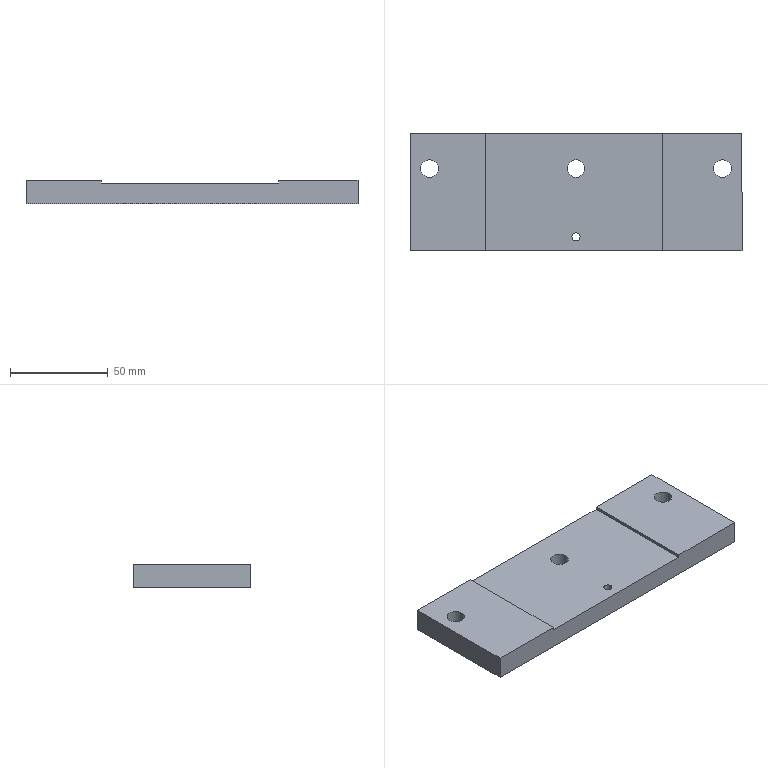Part | SolidWorks | features ICE 2, 3DProfileFeature 1, Extrusion 1, HoleWzd 1 | 1 solid | 20 faces | box 170 x 60 x 12 mm | volume 111868 mm3 | plane 10 | cylinder 8 | cone 2 | commonest cylinder face diameters 9 x6 4.2 x2
STEP:
#1=CARTESIAN_POINT('',(2.1,-23.,-5.575));
#2=VERTEX_POINT('',#1);
#3=CARTESIAN_POINT('',(-2.1,-23.,-5.575));
#4=VERTEX_POINT('',#3);
#5=CARTESIAN_POINT('',(0.,-23.,-5.575));
#6=DIRECTION('',(0.,0.,-1.));
#7=DIRECTION('',(-1.,0.,0.));
#8=AXIS2_PLACEMENT_3D('',#5,#6,#7);
#9=CIRCLE('',#8,2.1);
#10=EDGE_CURVE('',#2,#4,#9,.T.);
#11=ORIENTED_EDGE('',*,*,#10,.F.);
#12=CARTESIAN_POINT('',(2.525,-23.,-6.));
#13=VERTEX_POINT('',#12);
#14=CARTESIAN_POINT('',(2.525,-23.,-6.));
#15=DIRECTION('',(0.7071,0.,-0.7071));
#16=VECTOR('',#15,1000.);
#17=LINE('',#14,#16);
#18=EDGE_CURVE('',#2,#13,#17,.T.);
#19=ORIENTED_EDGE('',*,*,#18,.T.);
#20=CARTESIAN_POINT('',(-2.525,-23.,-6.));
#21=VERTEX_POINT('',#20);
#22=CARTESIAN_POINT('',(0.,-23.,-6.));
#23=DIRECTION('',(0.,0.,-1.));
#24=DIRECTION('',(-1.,0.,0.));
#25=AXIS2_PLACEMENT_3D('',#22,#23,#24);
#26=CIRCLE('',#25,2.525);
#27=EDGE_CURVE('',#13,#21,#26,.T.);
#28=ORIENTED_EDGE('',*,*,#27,.T.);
#29=CARTESIAN_POINT('',(-2.525,-23.,-6.));
#30=DIRECTION('',(-0.7071,0.,-0.7071));
#31=VECTOR('',#30,1000.);
#32=LINE('',#29,#31);
#33=EDGE_CURVE('',#4,#21,#32,.T.);
#34=ORIENTED_EDGE('',*,*,#33,.F.);
#35=EDGE_LOOP('',(#11,#19,#28,#34));
#36=FACE_OUTER_BOUND('',#35,.T.);
#37=CARTESIAN_POINT('',(0.,-23.,-6.));
#38=DIRECTION('',(0.,0.,-1.));
#39=DIRECTION('',(-1.,0.,0.));
#40=AXIS2_PLACEMENT_3D('',#37,#38,#39);
#41=CONICAL_SURFACE('',#40,2.525,0.7854);
#42=ADVANCED_FACE('',(#36),#41,.F.);
#43=CARTESIAN_POINT('',(2.1,-23.,4.5));
#44=VERTEX_POINT('',#43);
#45=CARTESIAN_POINT('',(-2.1,-23.,4.5));
#46=VERTEX_POINT('',#45);
#47=CARTESIAN_POINT('',(0.,-23.,4.5));
#48=DIRECTION('',(0.,0.,-1.));
#49=DIRECTION('',(-1.,0.,0.));
#50=AXIS2_PLACEMENT_3D('',#47,#48,#49);
#51=CIRCLE('',#50,2.1);
#52=EDGE_CURVE('',#44,#46,#51,.T.);
#53=ORIENTED_EDGE('',*,*,#52,.F.);
#54=CARTESIAN_POINT('',(2.1,-23.,-6.));
#55=DIRECTION('',(0.,0.,-1.));
#56=VECTOR('',#55,1000.);
#57=LINE('',#54,#56);
#58=EDGE_CURVE('',#44,#2,#57,.T.);
#59=ORIENTED_EDGE('',*,*,#58,.T.);
#60=ORIENTED_EDGE('',*,*,#10,.T.);
#61=CARTESIAN_POINT('',(-2.1,-23.,-6.));
#62=DIRECTION('',(0.,0.,-1.));
#63=VECTOR('',#62,1000.);
#64=LINE('',#61,#63);
#65=EDGE_CURVE('',#46,#4,#64,.T.);
#66=ORIENTED_EDGE('',*,*,#65,.F.);
#67=EDGE_LOOP('',(#53,#59,#60,#66));
#68=FACE_OUTER_BOUND('',#67,.T.);
#69=CARTESIAN_POINT('',(0.,-23.,-6.));
#70=DIRECTION('',(0.,0.,-1.));
#71=DIRECTION('',(-1.,0.,0.));
#72=AXIS2_PLACEMENT_3D('',#69,#70,#71);
#73=CYLINDRICAL_SURFACE('',#72,2.1);
#74=ADVANCED_FACE('',(#68),#73,.F.);
#75=CARTESIAN_POINT('',(4.5,12.,4.5));
#76=VERTEX_POINT('',#75);
#77=CARTESIAN_POINT('',(-4.5,12.,4.5));
#78=VERTEX_POINT('',#77);
#79=CARTESIAN_POINT('',(0.,12.,4.5));
#80=DIRECTION('',(0.,0.,-1.));
#81=DIRECTION('',(-1.,0.,0.));
#82=AXIS2_PLACEMENT_3D('',#79,#80,#81);
#83=CIRCLE('',#82,4.5);
#84=EDGE_CURVE('',#76,#78,#83,.T.);
#85=ORIENTED_EDGE('',*,*,#84,.F.);
#86=CARTESIAN_POINT('',(4.5,12.,-6.));
#87=VERTEX_POINT('',#86);
#88=CARTESIAN_POINT('',(4.5,12.,6.));
#89=DIRECTION('',(0.,0.,-1.));
#90=VECTOR('',#89,1000.);
#91=LINE('',#88,#90);
#92=EDGE_CURVE('',#76,#87,#91,.T.);
#93=ORIENTED_EDGE('',*,*,#92,.T.);
#94=CARTESIAN_POINT('',(-4.5,12.,-6.));
#95=VERTEX_POINT('',#94);
#96=CARTESIAN_POINT('',(0.,12.,-6.));
#97=DIRECTION('',(0.,0.,1.));
#98=DIRECTION('',(1.,0.,0.));
#99=AXIS2_PLACEMENT_3D('',#96,#97,#98);
#100=CIRCLE('',#99,4.5);
#101=EDGE_CURVE('',#95,#87,#100,.T.);
#102=ORIENTED_EDGE('',*,*,#101,.F.);
#103=CARTESIAN_POINT('',(-4.5,12.,6.));
#104=DIRECTION('',(0.,0.,-1.));
#105=VECTOR('',#104,1000.);
#106=LINE('',#103,#105);
#107=EDGE_CURVE('',#78,#95,#106,.T.);
#108=ORIENTED_EDGE('',*,*,#107,.F.);
#109=EDGE_LOOP('',(#85,#93,#102,#108));
#110=FACE_OUTER_BOUND('',#109,.T.);
#111=CARTESIAN_POINT('',(0.,12.,6.));
#112=DIRECTION('',(0.,0.,-1.));
#113=DIRECTION('',(-1.,0.,0.));
#114=AXIS2_PLACEMENT_3D('',#111,#112,#113);
#115=CYLINDRICAL_SURFACE('',#114,4.5);
#116=ADVANCED_FACE('',(#110),#115,.F.);
#117=CARTESIAN_POINT('',(70.5,12.,6.));
#118=VERTEX_POINT('',#117);
#119=CARTESIAN_POINT('',(79.5,12.,6.));
#120=VERTEX_POINT('',#119);
#121=CARTESIAN_POINT('',(75.,12.,6.));
#122=DIRECTION('',(0.,0.,1.));
#123=DIRECTION('',(1.,0.,0.));
#124=AXIS2_PLACEMENT_3D('',#121,#122,#123);
#125=CIRCLE('',#124,4.5);
#126=EDGE_CURVE('',#118,#120,#125,.T.);
#127=ORIENTED_EDGE('',*,*,#126,.T.);
#128=CARTESIAN_POINT('',(79.5,12.,-6.));
#129=VERTEX_POINT('',#128);
#130=CARTESIAN_POINT('',(79.5,12.,6.));
#131=DIRECTION('',(0.,0.,-1.));
#132=VECTOR('',#131,1000.);
#133=LINE('',#130,#132);
#134=EDGE_CURVE('',#120,#129,#133,.T.);
#135=ORIENTED_EDGE('',*,*,#134,.T.);
#136=CARTESIAN_POINT('',(70.5,12.,-6.));
#137=VERTEX_POINT('',#136);
#138=CARTESIAN_POINT('',(75.,12.,-6.));
#139=DIRECTION('',(0.,0.,1.));
#140=DIRECTION('',(1.,0.,0.));
#141=AXIS2_PLACEMENT_3D('',#138,#139,#140);
#142=CIRCLE('',#141,4.5);
#143=EDGE_CURVE('',#137,#129,#142,.T.);
#144=ORIENTED_EDGE('',*,*,#143,.F.);
#145=CARTESIAN_POINT('',(70.5,12.,6.));
#146=DIRECTION('',(0.,0.,-1.));
#147=VECTOR('',#146,1000.);
#148=LINE('',#145,#147);
#149=EDGE_CURVE('',#118,#137,#148,.T.);
#150=ORIENTED_EDGE('',*,*,#149,.F.);
#151=EDGE_LOOP('',(#127,#135,#144,#150));
#152=FACE_OUTER_BOUND('',#151,.T.);
#153=CARTESIAN_POINT('',(75.,12.,6.));
#154=DIRECTION('',(0.,0.,-1.));
#155=DIRECTION('',(-1.,0.,0.));
#156=AXIS2_PLACEMENT_3D('',#153,#154,#155);
#157=CYLINDRICAL_SURFACE('',#156,4.5);
#158=ADVANCED_FACE('',(#152),#157,.F.);
#159=CARTESIAN_POINT('',(-79.5,12.,6.));
#160=VERTEX_POINT('',#159);
#161=CARTESIAN_POINT('',(-70.5,12.,6.));
#162=VERTEX_POINT('',#161);
#163=CARTESIAN_POINT('',(-75.,12.,6.));
#164=DIRECTION('',(0.,0.,1.));
#165=DIRECTION('',(1.,0.,0.));
#166=AXIS2_PLACEMENT_3D('',#163,#164,#165);
#167=CIRCLE('',#166,4.5);
#168=EDGE_CURVE('',#160,#162,#167,.T.);
#169=ORIENTED_EDGE('',*,*,#168,.T.);
#170=CARTESIAN_POINT('',(-70.5,12.,-6.));
#171=VERTEX_POINT('',#170);
#172=CARTESIAN_POINT('',(-70.5,12.,6.));
#173=DIRECTION('',(0.,0.,-1.));
#174=VECTOR('',#173,1000.);
#175=LINE('',#172,#174);
#176=EDGE_CURVE('',#162,#171,#175,.T.);
#177=ORIENTED_EDGE('',*,*,#176,.T.);
#178=CARTESIAN_POINT('',(-79.5,12.,-6.));
#179=VERTEX_POINT('',#178);
#180=CARTESIAN_POINT('',(-75.,12.,-6.));
#181=DIRECTION('',(0.,0.,1.));
#182=DIRECTION('',(1.,0.,0.));
#183=AXIS2_PLACEMENT_3D('',#180,#181,#182);
#184=CIRCLE('',#183,4.5);
#185=EDGE_CURVE('',#179,#171,#184,.T.);
#186=ORIENTED_EDGE('',*,*,#185,.F.);
#187=CARTESIAN_POINT('',(-79.5,12.,6.));
#188=DIRECTION('',(0.,0.,-1.));
#189=VECTOR('',#188,1000.);
#190=LINE('',#187,#189);
#191=EDGE_CURVE('',#160,#179,#190,.T.);
#192=ORIENTED_EDGE('',*,*,#191,.F.);
#193=EDGE_LOOP('',(#169,#177,#186,#192));
#194=FACE_OUTER_BOUND('',#193,.T.);
#195=CARTESIAN_POINT('',(-75.,12.,6.));
#196=DIRECTION('',(0.,0.,-1.));
#197=DIRECTION('',(-1.,0.,0.));
#198=AXIS2_PLACEMENT_3D('',#195,#196,#197);
#199=CYLINDRICAL_SURFACE('',#198,4.5);
#200=ADVANCED_FACE('',(#194),#199,.F.);
#201=ORIENTED_EDGE('',*,*,#126,.F.);
#202=CARTESIAN_POINT('',(75.,12.,6.));
#203=DIRECTION('',(0.,0.,1.));
#204=DIRECTION('',(1.,0.,0.));
#205=AXIS2_PLACEMENT_3D('',#202,#203,#204);
#206=CIRCLE('',#205,4.5);
#207=EDGE_CURVE('',#120,#118,#206,.T.);
#208=ORIENTED_EDGE('',*,*,#207,.F.);
#209=EDGE_LOOP('',(#201,#208));
#210=FACE_BOUND('',#209,.T.);
#211=CARTESIAN_POINT('',(85.,30.,6.));
#212=VERTEX_POINT('',#211);
#213=CARTESIAN_POINT('',(44.5,30.,6.));
#214=VERTEX_POINT('',#213);
#215=CARTESIAN_POINT('',(-85.,30.,6.));
#216=DIRECTION('',(-1.,0.,0.));
#217=VECTOR('',#216,1000.);
#218=LINE('',#215,#217);
#219=EDGE_CURVE('',#212,#214,#218,.T.);
#220=ORIENTED_EDGE('',*,*,#219,.T.);
#221=CARTESIAN_POINT('',(44.5,-30.,6.));
#222=VERTEX_POINT('',#221);
#223=CARTESIAN_POINT('',(44.5,30.,6.));
#224=DIRECTION('',(0.,1.,0.));
#225=VECTOR('',#224,1000.);
#226=LINE('',#223,#225);
#227=EDGE_CURVE('',#222,#214,#226,.T.);
#228=ORIENTED_EDGE('',*,*,#227,.F.);
#229=CARTESIAN_POINT('',(85.,-30.,6.));
#230=VERTEX_POINT('',#229);
#231=CARTESIAN_POINT('',(-85.,-30.,6.));
#232=DIRECTION('',(1.,0.,0.));
#233=VECTOR('',#232,1000.);
#234=LINE('',#231,#233);
#235=EDGE_CURVE('',#222,#230,#234,.T.);
#236=ORIENTED_EDGE('',*,*,#235,.T.);
#237=CARTESIAN_POINT('',(85.,-30.,6.));
#238=DIRECTION('',(0.,1.,0.));
#239=VECTOR('',#238,1000.);
#240=LINE('',#237,#239);
#241=EDGE_CURVE('',#230,#212,#240,.T.);
#242=ORIENTED_EDGE('',*,*,#241,.T.);
#243=EDGE_LOOP('',(#220,#228,#236,#242));
#244=FACE_OUTER_BOUND('',#243,.T.);
#245=CARTESIAN_POINT('',(0.,0.,6.));
#246=DIRECTION('',(0.,0.,-1.));
#247=DIRECTION('',(-1.,0.,0.));
#248=AXIS2_PLACEMENT_3D('',#245,#246,#247);
#249=PLANE('',#248);
#250=ADVANCED_FACE('',(#210,#244),#249,.F.);
#251=CARTESIAN_POINT('',(-85.,-30.,6.));
#252=VERTEX_POINT('',#251);
#253=CARTESIAN_POINT('',(-46.5,-30.,6.));
#254=VERTEX_POINT('',#253);
#255=CARTESIAN_POINT('',(-85.,-30.,6.));
#256=DIRECTION('',(1.,0.,0.));
#257=VECTOR('',#256,1000.);
#258=LINE('',#255,#257);
#259=EDGE_CURVE('',#252,#254,#258,.T.);
#260=ORIENTED_EDGE('',*,*,#259,.T.);
#261=CARTESIAN_POINT('',(-46.5,30.,6.));
#262=VERTEX_POINT('',#261);
#263=CARTESIAN_POINT('',(-46.5,30.,6.));
#264=DIRECTION('',(0.,-1.,0.));
#265=VECTOR('',#264,1000.);
#266=LINE('',#263,#265);
#267=EDGE_CURVE('',#262,#254,#266,.T.);
#268=ORIENTED_EDGE('',*,*,#267,.F.);
#269=CARTESIAN_POINT('',(-85.,30.,6.));
#270=VERTEX_POINT('',#269);
#271=CARTESIAN_POINT('',(-85.,30.,6.));
#272=DIRECTION('',(-1.,0.,0.));
#273=VECTOR('',#272,1000.);
#274=LINE('',#271,#273);
#275=EDGE_CURVE('',#262,#270,#274,.T.);
#276=ORIENTED_EDGE('',*,*,#275,.T.);
#277=CARTESIAN_POINT('',(-85.,-30.,6.));
#278=DIRECTION('',(0.,-1.,0.));
#279=VECTOR('',#278,1000.);
#280=LINE('',#277,#279);
#281=EDGE_CURVE('',#270,#252,#280,.T.);
#282=ORIENTED_EDGE('',*,*,#281,.T.);
#283=EDGE_LOOP('',(#260,#268,#276,#282));
#284=FACE_OUTER_BOUND('',#283,.T.);
#285=ORIENTED_EDGE('',*,*,#168,.F.);
#286=CARTESIAN_POINT('',(-75.,12.,6.));
#287=DIRECTION('',(0.,0.,1.));
#288=DIRECTION('',(1.,0.,0.));
#289=AXIS2_PLACEMENT_3D('',#286,#287,#288);
#290=CIRCLE('',#289,4.5);
#291=EDGE_CURVE('',#162,#160,#290,.T.);
#292=ORIENTED_EDGE('',*,*,#291,.F.);
#293=EDGE_LOOP('',(#285,#292));
#294=FACE_BOUND('',#293,.T.);
#295=CARTESIAN_POINT('',(0.,0.,6.));
#296=DIRECTION('',(0.,0.,-1.));
#297=DIRECTION('',(-1.,0.,0.));
#298=AXIS2_PLACEMENT_3D('',#295,#296,#297);
#299=PLANE('',#298);
#300=ADVANCED_FACE('',(#284,#294),#299,.F.);
#301=CARTESIAN_POINT('',(0.,-23.,-6.));
#302=DIRECTION('',(0.,0.,-1.));
#303=DIRECTION('',(-1.,0.,0.));
#304=AXIS2_PLACEMENT_3D('',#301,#302,#303);
#305=CIRCLE('',#304,2.525);
#306=EDGE_CURVE('',#21,#13,#305,.T.);
#307=ORIENTED_EDGE('',*,*,#306,.F.);
#308=ORIENTED_EDGE('',*,*,#27,.F.);
#309=EDGE_LOOP('',(#307,#308));
#310=FACE_BOUND('',#309,.T.);
#311=ORIENTED_EDGE('',*,*,#143,.T.);
#312=CARTESIAN_POINT('',(75.,12.,-6.));
#313=DIRECTION('',(0.,0.,1.));
#314=DIRECTION('',(1.,0.,0.));
#315=AXIS2_PLACEMENT_3D('',#312,#313,#314);
#316=CIRCLE('',#315,4.5);
#317=EDGE_CURVE('',#129,#137,#316,.T.);
#318=ORIENTED_EDGE('',*,*,#317,.T.);
#319=EDGE_LOOP('',(#311,#318));
#320=FACE_BOUND('',#319,.T.);
#321=CARTESIAN_POINT('',(85.,-30.,-6.));
#322=VERTEX_POINT('',#321);
#323=CARTESIAN_POINT('',(85.,30.,-6.));
#324=VERTEX_POINT('',#323);
#325=CARTESIAN_POINT('',(85.,-30.,-6.));
#326=DIRECTION('',(0.,1.,0.));
#327=VECTOR('',#326,1000.);
#328=LINE('',#325,#327);
#329=EDGE_CURVE('',#322,#324,#328,.T.);
#330=ORIENTED_EDGE('',*,*,#329,.F.);
#331=CARTESIAN_POINT('',(-85.,-30.,-6.));
#332=VERTEX_POINT('',#331);
#333=CARTESIAN_POINT('',(-85.,-30.,-6.));
#334=DIRECTION('',(1.,0.,0.));
#335=VECTOR('',#334,1000.);
#336=LINE('',#333,#335);
#337=EDGE_CURVE('',#332,#322,#336,.T.);
#338=ORIENTED_EDGE('',*,*,#337,.F.);
#339=CARTESIAN_POINT('',(-85.,30.,-6.));
#340=VERTEX_POINT('',#339);
#341=CARTESIAN_POINT('',(-85.,-30.,-6.));
#342=DIRECTION('',(0.,-1.,0.));
#343=VECTOR('',#342,1000.);
#344=LINE('',#341,#343);
#345=EDGE_CURVE('',#340,#332,#344,.T.);
#346=ORIENTED_EDGE('',*,*,#345,.F.);
#347=CARTESIAN_POINT('',(-85.,30.,-6.));
#348=DIRECTION('',(-1.,0.,0.));
#349=VECTOR('',#348,1000.);
#350=LINE('',#347,#349);
#351=EDGE_CURVE('',#324,#340,#350,.T.);
#352=ORIENTED_EDGE('',*,*,#351,.F.);
#353=EDGE_LOOP('',(#330,#338,#346,#352));
#354=FACE_OUTER_BOUND('',#353,.T.);
#355=ORIENTED_EDGE('',*,*,#185,.T.);
#356=CARTESIAN_POINT('',(-75.,12.,-6.));
#357=DIRECTION('',(0.,0.,1.));
#358=DIRECTION('',(1.,0.,0.));
#359=AXIS2_PLACEMENT_3D('',#356,#357,#358);
#360=CIRCLE('',#359,4.5);
#361=EDGE_CURVE('',#171,#179,#360,.T.);
#362=ORIENTED_EDGE('',*,*,#361,.T.);
#363=EDGE_LOOP('',(#355,#362));
#364=FACE_BOUND('',#363,.T.);
#365=ORIENTED_EDGE('',*,*,#101,.T.);
#366=CARTESIAN_POINT('',(0.,12.,-6.));
#367=DIRECTION('',(0.,0.,1.));
#368=DIRECTION('',(1.,0.,0.));
#369=AXIS2_PLACEMENT_3D('',#366,#367,#368);
#370=CIRCLE('',#369,4.5);
#371=EDGE_CURVE('',#87,#95,#370,.T.);
#372=ORIENTED_EDGE('',*,*,#371,.T.);
#373=EDGE_LOOP('',(#365,#372));
#374=FACE_BOUND('',#373,.T.);
#375=CARTESIAN_POINT('',(0.,0.,-6.));
#376=DIRECTION('',(0.,0.,-1.));
#377=DIRECTION('',(-1.,0.,0.));
#378=AXIS2_PLACEMENT_3D('',#375,#376,#377);
#379=PLANE('',#378);
#380=ADVANCED_FACE('',(#310,#320,#354,#364,#374),#379,.T.);
#381=ORIENTED_EDGE('',*,*,#329,.T.);
#382=CARTESIAN_POINT('',(85.,30.,6.));
#383=DIRECTION('',(0.,0.,-1.));
#384=VECTOR('',#383,1000.);
#385=LINE('',#382,#384);
#386=EDGE_CURVE('',#212,#324,#385,.T.);
#387=ORIENTED_EDGE('',*,*,#386,.F.);
#388=ORIENTED_EDGE('',*,*,#241,.F.);
#389=CARTESIAN_POINT('',(85.,-30.,6.));
#390=DIRECTION('',(0.,0.,-1.));
#391=VECTOR('',#390,1000.);
#392=LINE('',#389,#391);
#393=EDGE_CURVE('',#230,#322,#392,.T.);
#394=ORIENTED_EDGE('',*,*,#393,.T.);
#395=EDGE_LOOP('',(#381,#387,#388,#394));
#396=FACE_OUTER_BOUND('',#395,.T.);
#397=CARTESIAN_POINT('',(85.,-30.,6.));
#398=DIRECTION('',(-1.,0.,0.));
#399=DIRECTION('',(0.,-1.,0.));
#400=AXIS2_PLACEMENT_3D('',#397,#398,#399);
#401=PLANE('',#400);
#402=ADVANCED_FACE('',(#396),#401,.F.);
#403=CARTESIAN_POINT('',(44.5,30.,4.5));
#404=VERTEX_POINT('',#403);
#405=CARTESIAN_POINT('',(-46.5,30.,4.5));
#406=VERTEX_POINT('',#405);
#407=CARTESIAN_POINT('',(44.5,30.,4.5));
#408=DIRECTION('',(-1.,0.,0.));
#409=VECTOR('',#408,1000.);
#410=LINE('',#407,#409);
#411=EDGE_CURVE('',#404,#406,#410,.T.);
#412=ORIENTED_EDGE('',*,*,#411,.F.);
#413=CARTESIAN_POINT('',(44.5,30.,4.5));
#414=DIRECTION('',(0.,0.,1.));
#415=VECTOR('',#414,1000.);
#416=LINE('',#413,#415);
#417=EDGE_CURVE('',#404,#214,#416,.T.);
#418=ORIENTED_EDGE('',*,*,#417,.T.);
#419=ORIENTED_EDGE('',*,*,#219,.F.);
#420=ORIENTED_EDGE('',*,*,#386,.T.);
#421=ORIENTED_EDGE('',*,*,#351,.T.);
#422=CARTESIAN_POINT('',(-85.,30.,6.));
#423=DIRECTION('',(0.,0.,-1.));
#424=VECTOR('',#423,1000.);
#425=LINE('',#422,#424);
#426=EDGE_CURVE('',#270,#340,#425,.T.);
#427=ORIENTED_EDGE('',*,*,#426,.F.);
#428=ORIENTED_EDGE('',*,*,#275,.F.);
#429=CARTESIAN_POINT('',(-46.5,30.,4.5));
#430=DIRECTION('',(0.,0.,1.));
#431=VECTOR('',#430,1000.);
#432=LINE('',#429,#431);
#433=EDGE_CURVE('',#406,#262,#432,.T.);
#434=ORIENTED_EDGE('',*,*,#433,.F.);
#435=EDGE_LOOP('',(#412,#418,#419,#420,#421,#427,#428,#434));
#436=FACE_OUTER_BOUND('',#435,.T.);
#437=CARTESIAN_POINT('',(-85.,30.,6.));
#438=DIRECTION('',(0.,-1.,0.));
#439=DIRECTION('',(0.,0.,-1.));
#440=AXIS2_PLACEMENT_3D('',#437,#438,#439);
#441=PLANE('',#440);
#442=ADVANCED_FACE('',(#436),#441,.F.);
#443=ORIENTED_EDGE('',*,*,#345,.T.);
#444=CARTESIAN_POINT('',(-85.,-30.,6.));
#445=DIRECTION('',(0.,0.,-1.));
#446=VECTOR('',#445,1000.);
#447=LINE('',#444,#446);
#448=EDGE_CURVE('',#252,#332,#447,.T.);
#449=ORIENTED_EDGE('',*,*,#448,.F.);
#450=ORIENTED_EDGE('',*,*,#281,.F.);
#451=ORIENTED_EDGE('',*,*,#426,.T.);
#452=EDGE_LOOP('',(#443,#449,#450,#451));
#453=FACE_OUTER_BOUND('',#452,.T.);
#454=CARTESIAN_POINT('',(-85.,-30.,6.));
#455=DIRECTION('',(1.,0.,0.));
#456=DIRECTION('',(0.,0.,-1.));
#457=AXIS2_PLACEMENT_3D('',#454,#455,#456);
#458=PLANE('',#457);
#459=ADVANCED_FACE('',(#453),#458,.F.);
#460=ORIENTED_EDGE('',*,*,#235,.F.);
#461=CARTESIAN_POINT('',(44.5,-30.,4.5));
#462=VERTEX_POINT('',#461);
#463=CARTESIAN_POINT('',(44.5,-30.,4.5));
#464=DIRECTION('',(0.,0.,1.));
#465=VECTOR('',#464,1000.);
#466=LINE('',#463,#465);
#467=EDGE_CURVE('',#462,#222,#466,.T.);
#468=ORIENTED_EDGE('',*,*,#467,.F.);
#469=CARTESIAN_POINT('',(-46.5,-30.,4.5));
#470=VERTEX_POINT('',#469);
#471=CARTESIAN_POINT('',(44.5,-30.,4.5));
#472=DIRECTION('',(1.,0.,0.));
#473=VECTOR('',#472,1000.);
#474=LINE('',#471,#473);
#475=EDGE_CURVE('',#470,#462,#474,.T.);
#476=ORIENTED_EDGE('',*,*,#475,.F.);
#477=CARTESIAN_POINT('',(-46.5,-30.,4.5));
#478=DIRECTION('',(0.,0.,1.));
#479=VECTOR('',#478,1000.);
#480=LINE('',#477,#479);
#481=EDGE_CURVE('',#470,#254,#480,.T.);
#482=ORIENTED_EDGE('',*,*,#481,.T.);
#483=ORIENTED_EDGE('',*,*,#259,.F.);
#484=ORIENTED_EDGE('',*,*,#448,.T.);
#485=ORIENTED_EDGE('',*,*,#337,.T.);
#486=ORIENTED_EDGE('',*,*,#393,.F.);
#487=EDGE_LOOP('',(#460,#468,#476,#482,#483,#484,#485,#486));
#488=FACE_OUTER_BOUND('',#487,.T.);
#489=CARTESIAN_POINT('',(-85.,-30.,6.));
#490=DIRECTION('',(0.,1.,0.));
#491=DIRECTION('',(0.,0.,1.));
#492=AXIS2_PLACEMENT_3D('',#489,#490,#491);
#493=PLANE('',#492);
#494=ADVANCED_FACE('',(#488),#493,.F.);
#495=ORIENTED_EDGE('',*,*,#176,.F.);
#496=ORIENTED_EDGE('',*,*,#291,.T.);
#497=ORIENTED_EDGE('',*,*,#191,.T.);
#498=ORIENTED_EDGE('',*,*,#361,.F.);
#499=EDGE_LOOP('',(#495,#496,#497,#498));
#500=FACE_OUTER_BOUND('',#499,.T.);
#501=CARTESIAN_POINT('',(-75.,12.,6.));
#502=DIRECTION('',(0.,0.,-1.));
#503=DIRECTION('',(-1.,0.,0.));
#504=AXIS2_PLACEMENT_3D('',#501,#502,#503);
#505=CYLINDRICAL_SURFACE('',#504,4.5);
#506=ADVANCED_FACE('',(#500),#505,.F.);
#507=ORIENTED_EDGE('',*,*,#134,.F.);
#508=ORIENTED_EDGE('',*,*,#207,.T.);
#509=ORIENTED_EDGE('',*,*,#149,.T.);
#510=ORIENTED_EDGE('',*,*,#317,.F.);
#511=EDGE_LOOP('',(#507,#508,#509,#510));
#512=FACE_OUTER_BOUND('',#511,.T.);
#513=CARTESIAN_POINT('',(75.,12.,6.));
#514=DIRECTION('',(0.,0.,-1.));
#515=DIRECTION('',(-1.,0.,0.));
#516=AXIS2_PLACEMENT_3D('',#513,#514,#515);
#517=CYLINDRICAL_SURFACE('',#516,4.5);
#518=ADVANCED_FACE('',(#512),#517,.F.);
#519=ORIENTED_EDGE('',*,*,#92,.F.);
#520=CARTESIAN_POINT('',(0.,12.,4.5));
#521=DIRECTION('',(0.,0.,-1.));
#522=DIRECTION('',(-1.,0.,0.));
#523=AXIS2_PLACEMENT_3D('',#520,#521,#522);
#524=CIRCLE('',#523,4.5);
#525=EDGE_CURVE('',#78,#76,#524,.T.);
#526=ORIENTED_EDGE('',*,*,#525,.F.);
#527=ORIENTED_EDGE('',*,*,#107,.T.);
#528=ORIENTED_EDGE('',*,*,#371,.F.);
#529=EDGE_LOOP('',(#519,#526,#527,#528));
#530=FACE_OUTER_BOUND('',#529,.T.);
#531=CARTESIAN_POINT('',(0.,12.,6.));
#532=DIRECTION('',(0.,0.,-1.));
#533=DIRECTION('',(-1.,0.,0.));
#534=AXIS2_PLACEMENT_3D('',#531,#532,#533);
#535=CYLINDRICAL_SURFACE('',#534,4.5);
#536=ADVANCED_FACE('',(#530),#535,.F.);
#537=ORIENTED_EDGE('',*,*,#227,.T.);
#538=ORIENTED_EDGE('',*,*,#417,.F.);
#539=CARTESIAN_POINT('',(44.5,30.,4.5));
#540=DIRECTION('',(0.,1.,0.));
#541=VECTOR('',#540,1000.);
#542=LINE('',#539,#541);
#543=EDGE_CURVE('',#462,#404,#542,.T.);
#544=ORIENTED_EDGE('',*,*,#543,.F.);
#545=ORIENTED_EDGE('',*,*,#467,.T.);
#546=EDGE_LOOP('',(#537,#538,#544,#545));
#547=FACE_OUTER_BOUND('',#546,.T.);
#548=CARTESIAN_POINT('',(44.5,30.,4.5));
#549=DIRECTION('',(1.,0.,0.));
#550=DIRECTION('',(0.,1.,0.));
#551=AXIS2_PLACEMENT_3D('',#548,#549,#550);
#552=PLANE('',#551);
#553=ADVANCED_FACE('',(#547),#552,.F.);
#554=ORIENTED_EDGE('',*,*,#267,.T.);
#555=ORIENTED_EDGE('',*,*,#481,.F.);
#556=CARTESIAN_POINT('',(-46.5,30.,4.5));
#557=DIRECTION('',(0.,-1.,0.));
#558=VECTOR('',#557,1000.);
#559=LINE('',#556,#558);
#560=EDGE_CURVE('',#406,#470,#559,.T.);
#561=ORIENTED_EDGE('',*,*,#560,.F.);
#562=ORIENTED_EDGE('',*,*,#433,.T.);
#563=EDGE_LOOP('',(#554,#555,#561,#562));
#564=FACE_OUTER_BOUND('',#563,.T.);
#565=CARTESIAN_POINT('',(-46.5,30.,4.5));
#566=DIRECTION('',(-1.,0.,0.));
#567=DIRECTION('',(0.,0.,1.));
#568=AXIS2_PLACEMENT_3D('',#565,#566,#567);
#569=PLANE('',#568);
#570=ADVANCED_FACE('',(#564),#569,.F.);
#571=CARTESIAN_POINT('',(0.,-23.,4.5));
#572=DIRECTION('',(0.,0.,-1.));
#573=DIRECTION('',(-1.,0.,0.));
#574=AXIS2_PLACEMENT_3D('',#571,#572,#573);
#575=CIRCLE('',#574,2.1);
#576=EDGE_CURVE('',#46,#44,#575,.T.);
#577=ORIENTED_EDGE('',*,*,#576,.T.);
#578=ORIENTED_EDGE('',*,*,#52,.T.);
#579=EDGE_LOOP('',(#577,#578));
#580=FACE_BOUND('',#579,.T.);
#581=ORIENTED_EDGE('',*,*,#525,.T.);
#582=ORIENTED_EDGE('',*,*,#84,.T.);
#583=EDGE_LOOP('',(#581,#582));
#584=FACE_BOUND('',#583,.T.);
#585=ORIENTED_EDGE('',*,*,#543,.T.);
#586=ORIENTED_EDGE('',*,*,#411,.T.);
#587=ORIENTED_EDGE('',*,*,#560,.T.);
#588=ORIENTED_EDGE('',*,*,#475,.T.);
#589=EDGE_LOOP('',(#585,#586,#587,#588));
#590=FACE_OUTER_BOUND('',#589,.T.);
#591=CARTESIAN_POINT('',(0.,0.,4.5));
#592=DIRECTION('',(0.,0.,-1.));
#593=DIRECTION('',(-1.,0.,0.));
#594=AXIS2_PLACEMENT_3D('',#591,#592,#593);
#595=PLANE('',#594);
#596=ADVANCED_FACE('',(#580,#584,#590),#595,.F.);
#597=ORIENTED_EDGE('',*,*,#58,.F.);
#598=ORIENTED_EDGE('',*,*,#576,.F.);
#599=ORIENTED_EDGE('',*,*,#65,.T.);
#600=CARTESIAN_POINT('',(0.,-23.,-5.575));
#601=DIRECTION('',(0.,0.,-1.));
#602=DIRECTION('',(-1.,0.,0.));
#603=AXIS2_PLACEMENT_3D('',#600,#601,#602);
#604=CIRCLE('',#603,2.1);
#605=EDGE_CURVE('',#4,#2,#604,.T.);
#606=ORIENTED_EDGE('',*,*,#605,.T.);
#607=EDGE_LOOP('',(#597,#598,#599,#606));
#608=FACE_OUTER_BOUND('',#607,.T.);
#609=CARTESIAN_POINT('',(0.,-23.,-6.));
#610=DIRECTION('',(0.,0.,-1.));
#611=DIRECTION('',(-1.,0.,0.));
#612=AXIS2_PLACEMENT_3D('',#609,#610,#611);
#613=CYLINDRICAL_SURFACE('',#612,2.1);
#614=ADVANCED_FACE('',(#608),#613,.F.);
#615=ORIENTED_EDGE('',*,*,#18,.F.);
#616=ORIENTED_EDGE('',*,*,#605,.F.);
#617=ORIENTED_EDGE('',*,*,#33,.T.);
#618=ORIENTED_EDGE('',*,*,#306,.T.);
#619=EDGE_LOOP('',(#615,#616,#617,#618));
#620=FACE_OUTER_BOUND('',#619,.T.);
#621=CARTESIAN_POINT('',(0.,-23.,-6.));
#622=DIRECTION('',(0.,0.,-1.));
#623=DIRECTION('',(-1.,0.,0.));
#624=AXIS2_PLACEMENT_3D('',#621,#622,#623);
#625=CONICAL_SURFACE('',#624,2.525,0.7854);
#626=ADVANCED_FACE('',(#620),#625,.F.);
#627=CLOSED_SHELL('',(#42,#74,#116,#158,#200,#250,#300,#380,#402,#442,#459,#494,#506,#518,#536,#553,#570,#596,#614,#626));
#628=MANIFOLD_SOLID_BREP('',#627);
#629=CARTESIAN_POINT('',(0.,0.,0.));
#630=DIRECTION('',(0.,0.,1.));
#631=DIRECTION('',(1.,0.,0.));
#632=AXIS2_PLACEMENT_3D('',#629,#630,#631);
#633=(LENGTH_UNIT()NAMED_UNIT(*)SI_UNIT(.MILLI.,.METRE.));
#634=UNCERTAINTY_MEASURE_WITH_UNIT(LENGTH_MEASURE(0.00001),#633,'','');
#635=(NAMED_UNIT(*)PLANE_ANGLE_UNIT()SI_UNIT($,.RADIAN.));
#636=(NAMED_UNIT(*)SI_UNIT($,.STERADIAN.)SOLID_ANGLE_UNIT());
#637=(GEOMETRIC_REPRESENTATION_CONTEXT(3)GLOBAL_UNCERTAINTY_ASSIGNED_CONTEXT((#634))GLOBAL_UNIT_ASSIGNED_CONTEXT((#633,#635,#636))REPRESENTATION_CONTEXT('',''));
#638=ADVANCED_BREP_SHAPE_REPRESENTATION('',(#628,#632),#637);